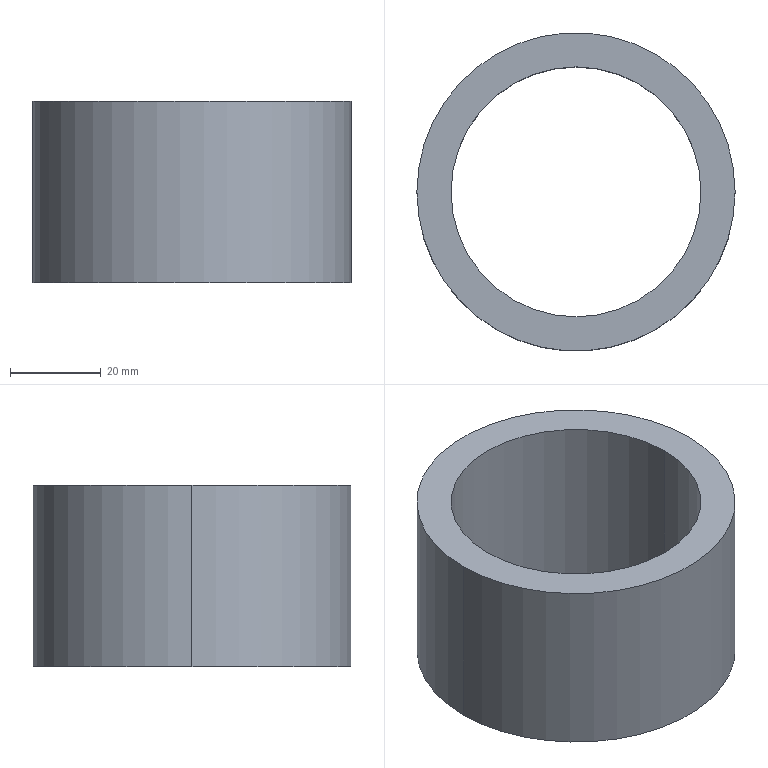Part | SolidWorks | features Extrusion 1 | 1 solid | 6 faces | box 70 x 70 x 40 mm | volume 58905 mm3 | cylinder 4 | plane 2 | commonest cylinder face diameters 55 x2 70 x2
STEP:
#1=CARTESIAN_POINT('',(-27.5,0.,40.));
#2=VERTEX_POINT('',#1);
#3=CARTESIAN_POINT('',(27.5,0.,40.));
#4=VERTEX_POINT('',#3);
#5=CARTESIAN_POINT('',(0.,0.,40.));
#6=DIRECTION('',(0.,0.,1.));
#7=DIRECTION('',(1.,0.,0.));
#8=AXIS2_PLACEMENT_3D('',#5,#6,#7);
#9=CIRCLE('',#8,27.5);
#10=EDGE_CURVE('',#2,#4,#9,.T.);
#11=ORIENTED_EDGE('',*,*,#10,.T.);
#12=CARTESIAN_POINT('',(27.5,0.,0.));
#13=VERTEX_POINT('',#12);
#14=CARTESIAN_POINT('',(27.5,0.,40.));
#15=DIRECTION('',(0.,0.,-1.));
#16=VECTOR('',#15,1000.);
#17=LINE('',#14,#16);
#18=EDGE_CURVE('',#4,#13,#17,.T.);
#19=ORIENTED_EDGE('',*,*,#18,.T.);
#20=CARTESIAN_POINT('',(-27.5,0.,0.));
#21=VERTEX_POINT('',#20);
#22=CARTESIAN_POINT('',(0.,0.,0.));
#23=DIRECTION('',(0.,0.,1.));
#24=DIRECTION('',(1.,0.,0.));
#25=AXIS2_PLACEMENT_3D('',#22,#23,#24);
#26=CIRCLE('',#25,27.5);
#27=EDGE_CURVE('',#21,#13,#26,.T.);
#28=ORIENTED_EDGE('',*,*,#27,.F.);
#29=CARTESIAN_POINT('',(-27.5,0.,40.));
#30=DIRECTION('',(0.,0.,-1.));
#31=VECTOR('',#30,1000.);
#32=LINE('',#29,#31);
#33=EDGE_CURVE('',#2,#21,#32,.T.);
#34=ORIENTED_EDGE('',*,*,#33,.F.);
#35=EDGE_LOOP('',(#11,#19,#28,#34));
#36=FACE_OUTER_BOUND('',#35,.T.);
#37=CARTESIAN_POINT('',(0.,0.,40.));
#38=DIRECTION('',(0.,0.,-1.));
#39=DIRECTION('',(-1.,0.,0.));
#40=AXIS2_PLACEMENT_3D('',#37,#38,#39);
#41=CYLINDRICAL_SURFACE('',#40,27.5);
#42=ADVANCED_FACE('',(#36),#41,.F.);
#43=CARTESIAN_POINT('',(35.,0.,40.));
#44=VERTEX_POINT('',#43);
#45=CARTESIAN_POINT('',(-35.,0.,40.));
#46=VERTEX_POINT('',#45);
#47=CARTESIAN_POINT('',(0.,0.,40.));
#48=DIRECTION('',(0.,0.,1.));
#49=DIRECTION('',(1.,0.,0.));
#50=AXIS2_PLACEMENT_3D('',#47,#48,#49);
#51=CIRCLE('',#50,35.);
#52=EDGE_CURVE('',#44,#46,#51,.T.);
#53=ORIENTED_EDGE('',*,*,#52,.F.);
#54=CARTESIAN_POINT('',(35.,0.,0.));
#55=VERTEX_POINT('',#54);
#56=CARTESIAN_POINT('',(35.,0.,40.));
#57=DIRECTION('',(0.,0.,-1.));
#58=VECTOR('',#57,1000.);
#59=LINE('',#56,#58);
#60=EDGE_CURVE('',#44,#55,#59,.T.);
#61=ORIENTED_EDGE('',*,*,#60,.T.);
#62=CARTESIAN_POINT('',(-35.,0.,0.));
#63=VERTEX_POINT('',#62);
#64=CARTESIAN_POINT('',(0.,0.,0.));
#65=DIRECTION('',(0.,0.,1.));
#66=DIRECTION('',(1.,0.,0.));
#67=AXIS2_PLACEMENT_3D('',#64,#65,#66);
#68=CIRCLE('',#67,35.);
#69=EDGE_CURVE('',#55,#63,#68,.T.);
#70=ORIENTED_EDGE('',*,*,#69,.T.);
#71=CARTESIAN_POINT('',(-35.,0.,40.));
#72=DIRECTION('',(0.,0.,-1.));
#73=VECTOR('',#72,1000.);
#74=LINE('',#71,#73);
#75=EDGE_CURVE('',#46,#63,#74,.T.);
#76=ORIENTED_EDGE('',*,*,#75,.F.);
#77=EDGE_LOOP('',(#53,#61,#70,#76));
#78=FACE_OUTER_BOUND('',#77,.T.);
#79=CARTESIAN_POINT('',(0.,0.,40.));
#80=DIRECTION('',(0.,0.,-1.));
#81=DIRECTION('',(-1.,0.,0.));
#82=AXIS2_PLACEMENT_3D('',#79,#80,#81);
#83=CYLINDRICAL_SURFACE('',#82,35.);
#84=ADVANCED_FACE('',(#78),#83,.T.);
#85=CARTESIAN_POINT('',(0.,0.,40.));
#86=DIRECTION('',(0.,0.,1.));
#87=DIRECTION('',(1.,0.,0.));
#88=AXIS2_PLACEMENT_3D('',#85,#86,#87);
#89=CIRCLE('',#88,35.);
#90=EDGE_CURVE('',#46,#44,#89,.T.);
#91=ORIENTED_EDGE('',*,*,#90,.T.);
#92=ORIENTED_EDGE('',*,*,#52,.T.);
#93=EDGE_LOOP('',(#91,#92));
#94=FACE_OUTER_BOUND('',#93,.T.);
#95=ORIENTED_EDGE('',*,*,#10,.F.);
#96=CARTESIAN_POINT('',(0.,0.,40.));
#97=DIRECTION('',(0.,0.,1.));
#98=DIRECTION('',(1.,0.,0.));
#99=AXIS2_PLACEMENT_3D('',#96,#97,#98);
#100=CIRCLE('',#99,27.5);
#101=EDGE_CURVE('',#4,#2,#100,.T.);
#102=ORIENTED_EDGE('',*,*,#101,.F.);
#103=EDGE_LOOP('',(#95,#102));
#104=FACE_BOUND('',#103,.T.);
#105=CARTESIAN_POINT('',(0.,0.,40.));
#106=DIRECTION('',(0.,0.,1.));
#107=DIRECTION('',(1.,0.,0.));
#108=AXIS2_PLACEMENT_3D('',#105,#106,#107);
#109=PLANE('',#108);
#110=ADVANCED_FACE('',(#94,#104),#109,.T.);
#111=CARTESIAN_POINT('',(0.,0.,0.));
#112=DIRECTION('',(0.,0.,1.));
#113=DIRECTION('',(1.,0.,0.));
#114=AXIS2_PLACEMENT_3D('',#111,#112,#113);
#115=CIRCLE('',#114,35.);
#116=EDGE_CURVE('',#63,#55,#115,.T.);
#117=ORIENTED_EDGE('',*,*,#116,.F.);
#118=ORIENTED_EDGE('',*,*,#69,.F.);
#119=EDGE_LOOP('',(#117,#118));
#120=FACE_OUTER_BOUND('',#119,.T.);
#121=ORIENTED_EDGE('',*,*,#27,.T.);
#122=CARTESIAN_POINT('',(0.,0.,0.));
#123=DIRECTION('',(0.,0.,1.));
#124=DIRECTION('',(1.,0.,0.));
#125=AXIS2_PLACEMENT_3D('',#122,#123,#124);
#126=CIRCLE('',#125,27.5);
#127=EDGE_CURVE('',#13,#21,#126,.T.);
#128=ORIENTED_EDGE('',*,*,#127,.T.);
#129=EDGE_LOOP('',(#121,#128));
#130=FACE_BOUND('',#129,.T.);
#131=CARTESIAN_POINT('',(0.,0.,0.));
#132=DIRECTION('',(0.,0.,1.));
#133=DIRECTION('',(1.,0.,0.));
#134=AXIS2_PLACEMENT_3D('',#131,#132,#133);
#135=PLANE('',#134);
#136=ADVANCED_FACE('',(#120,#130),#135,.F.);
#137=ORIENTED_EDGE('',*,*,#60,.F.);
#138=ORIENTED_EDGE('',*,*,#90,.F.);
#139=ORIENTED_EDGE('',*,*,#75,.T.);
#140=ORIENTED_EDGE('',*,*,#116,.T.);
#141=EDGE_LOOP('',(#137,#138,#139,#140));
#142=FACE_OUTER_BOUND('',#141,.T.);
#143=CARTESIAN_POINT('',(0.,0.,40.));
#144=DIRECTION('',(0.,0.,-1.));
#145=DIRECTION('',(-1.,0.,0.));
#146=AXIS2_PLACEMENT_3D('',#143,#144,#145);
#147=CYLINDRICAL_SURFACE('',#146,35.);
#148=ADVANCED_FACE('',(#142),#147,.T.);
#149=ORIENTED_EDGE('',*,*,#18,.F.);
#150=ORIENTED_EDGE('',*,*,#101,.T.);
#151=ORIENTED_EDGE('',*,*,#33,.T.);
#152=ORIENTED_EDGE('',*,*,#127,.F.);
#153=EDGE_LOOP('',(#149,#150,#151,#152));
#154=FACE_OUTER_BOUND('',#153,.T.);
#155=CARTESIAN_POINT('',(0.,0.,40.));
#156=DIRECTION('',(0.,0.,-1.));
#157=DIRECTION('',(-1.,0.,0.));
#158=AXIS2_PLACEMENT_3D('',#155,#156,#157);
#159=CYLINDRICAL_SURFACE('',#158,27.5);
#160=ADVANCED_FACE('',(#154),#159,.F.);
#161=CLOSED_SHELL('',(#42,#84,#110,#136,#148,#160));
#162=MANIFOLD_SOLID_BREP('',#161);
#163=CARTESIAN_POINT('',(0.,0.,0.));
#164=DIRECTION('',(0.,0.,1.));
#165=DIRECTION('',(1.,0.,0.));
#166=AXIS2_PLACEMENT_3D('',#163,#164,#165);
#167=(LENGTH_UNIT()NAMED_UNIT(*)SI_UNIT(.MILLI.,.METRE.));
#168=UNCERTAINTY_MEASURE_WITH_UNIT(LENGTH_MEASURE(0.00001),#167,'','');
#169=(NAMED_UNIT(*)PLANE_ANGLE_UNIT()SI_UNIT($,.RADIAN.));
#170=(NAMED_UNIT(*)SI_UNIT($,.STERADIAN.)SOLID_ANGLE_UNIT());
#171=(GEOMETRIC_REPRESENTATION_CONTEXT(3)GLOBAL_UNCERTAINTY_ASSIGNED_CONTEXT((#168))GLOBAL_UNIT_ASSIGNED_CONTEXT((#167,#169,#170))REPRESENTATION_CONTEXT('',''));
#172=ADVANCED_BREP_SHAPE_REPRESENTATION('',(#162,#166),#171);